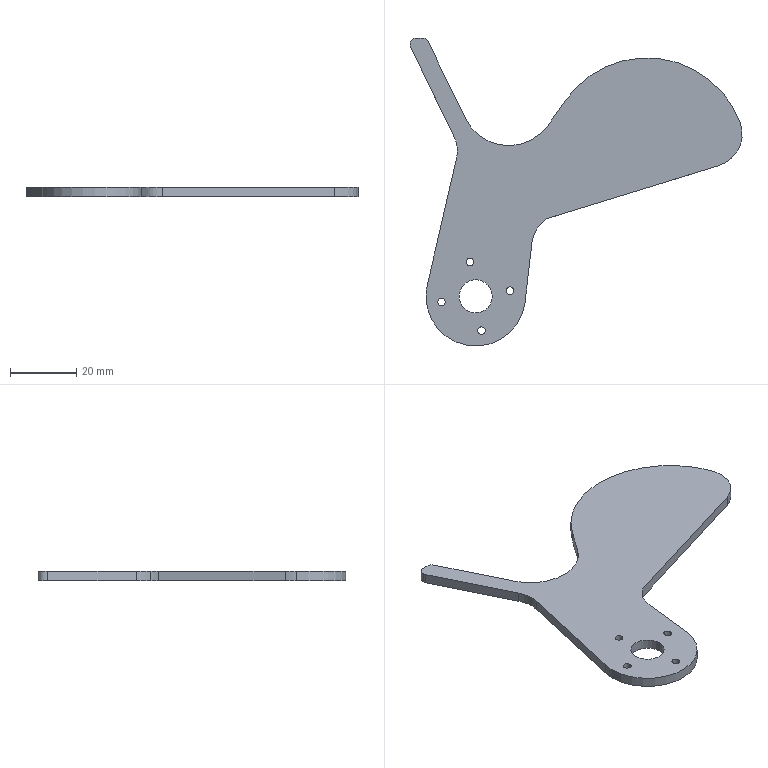Part | SolidWorks | features ICE 4, Fillet 2, BaseBody 1, HoleWzd 1 | 1 solid | 29 faces | box 100.288 x 93 x 3 mm | volume 11352 mm3 | cylinder 20 | plane 9 | commonest cylinder face diameters 2.3 x8 20 x4 4 x2 10 x2 30 x2 29 x1
STEP:
#1=CARTESIAN_POINT('',(-15.,-60.,0.));
#2=VERTEX_POINT('',#1);
#3=CARTESIAN_POINT('',(-5.,-60.,0.));
#4=VERTEX_POINT('',#3);
#5=CARTESIAN_POINT('',(-10.,-60.,0.));
#6=DIRECTION('',(0.,0.,1.));
#7=DIRECTION('',(1.,0.,0.));
#8=AXIS2_PLACEMENT_3D('',#5,#6,#7);
#9=CIRCLE('',#8,5.);
#10=EDGE_CURVE('',#2,#4,#9,.T.);
#11=ORIENTED_EDGE('',*,*,#10,.F.);
#12=CARTESIAN_POINT('',(-15.,-60.,3.));
#13=VERTEX_POINT('',#12);
#14=CARTESIAN_POINT('',(-15.,-60.,0.));
#15=DIRECTION('',(0.,0.,1.));
#16=VECTOR('',#15,1000.);
#17=LINE('',#14,#16);
#18=EDGE_CURVE('',#2,#13,#17,.T.);
#19=ORIENTED_EDGE('',*,*,#18,.T.);
#20=CARTESIAN_POINT('',(-5.,-60.,3.));
#21=VERTEX_POINT('',#20);
#22=CARTESIAN_POINT('',(-10.,-60.,3.));
#23=DIRECTION('',(0.,0.,1.));
#24=DIRECTION('',(1.,0.,0.));
#25=AXIS2_PLACEMENT_3D('',#22,#23,#24);
#26=CIRCLE('',#25,5.);
#27=EDGE_CURVE('',#13,#21,#26,.T.);
#28=ORIENTED_EDGE('',*,*,#27,.T.);
#29=CARTESIAN_POINT('',(-5.,-60.,0.));
#30=DIRECTION('',(0.,0.,1.));
#31=VECTOR('',#30,1000.);
#32=LINE('',#29,#31);
#33=EDGE_CURVE('',#4,#21,#32,.T.);
#34=ORIENTED_EDGE('',*,*,#33,.F.);
#35=EDGE_LOOP('',(#11,#19,#28,#34));
#36=FACE_OUTER_BOUND('',#35,.T.);
#37=CARTESIAN_POINT('',(-10.,-60.,0.));
#38=DIRECTION('',(0.,0.,1.));
#39=DIRECTION('',(1.,0.,0.));
#40=AXIS2_PLACEMENT_3D('',#37,#38,#39);
#41=CYLINDRICAL_SURFACE('',#40,5.);
#42=ADVANCED_FACE('',(#36),#41,.F.);
#43=CARTESIAN_POINT('',(-19.208,-61.722,0.));
#44=VERTEX_POINT('',#43);
#45=CARTESIAN_POINT('',(-21.508,-61.722,0.));
#46=VERTEX_POINT('',#45);
#47=CARTESIAN_POINT('',(-20.358,-61.722,0.));
#48=DIRECTION('',(0.,0.,-1.));
#49=DIRECTION('',(-1.,0.,0.));
#50=AXIS2_PLACEMENT_3D('',#47,#48,#49);
#51=CIRCLE('',#50,1.15);
#52=EDGE_CURVE('',#44,#46,#51,.T.);
#53=ORIENTED_EDGE('',*,*,#52,.T.);
#54=CARTESIAN_POINT('',(-21.508,-61.722,3.));
#55=VERTEX_POINT('',#54);
#56=CARTESIAN_POINT('',(-21.508,-61.722,3.));
#57=DIRECTION('',(0.,0.,1.));
#58=VECTOR('',#57,1000.);
#59=LINE('',#56,#58);
#60=EDGE_CURVE('',#46,#55,#59,.T.);
#61=ORIENTED_EDGE('',*,*,#60,.T.);
#62=CARTESIAN_POINT('',(-19.208,-61.722,3.));
#63=VERTEX_POINT('',#62);
#64=CARTESIAN_POINT('',(-20.358,-61.722,3.));
#65=DIRECTION('',(0.,0.,1.));
#66=DIRECTION('',(1.,0.,0.));
#67=AXIS2_PLACEMENT_3D('',#64,#65,#66);
#68=CIRCLE('',#67,1.15);
#69=EDGE_CURVE('',#55,#63,#68,.T.);
#70=ORIENTED_EDGE('',*,*,#69,.T.);
#71=CARTESIAN_POINT('',(-19.208,-61.722,3.));
#72=DIRECTION('',(0.,0.,1.));
#73=VECTOR('',#72,1000.);
#74=LINE('',#71,#73);
#75=EDGE_CURVE('',#44,#63,#74,.T.);
#76=ORIENTED_EDGE('',*,*,#75,.F.);
#77=EDGE_LOOP('',(#53,#61,#70,#76));
#78=FACE_OUTER_BOUND('',#77,.T.);
#79=CARTESIAN_POINT('',(-20.358,-61.722,3.));
#80=DIRECTION('',(0.,0.,1.));
#81=DIRECTION('',(1.,0.,0.));
#82=AXIS2_PLACEMENT_3D('',#79,#80,#81);
#83=CYLINDRICAL_SURFACE('',#82,1.15);
#84=ADVANCED_FACE('',(#78),#83,.F.);
#85=CARTESIAN_POINT('',(-10.572,-49.642,0.));
#86=VERTEX_POINT('',#85);
#87=CARTESIAN_POINT('',(-12.872,-49.642,0.));
#88=VERTEX_POINT('',#87);
#89=CARTESIAN_POINT('',(-11.722,-49.642,0.));
#90=DIRECTION('',(0.,0.,-1.));
#91=DIRECTION('',(-1.,0.,0.));
#92=AXIS2_PLACEMENT_3D('',#89,#90,#91);
#93=CIRCLE('',#92,1.15);
#94=EDGE_CURVE('',#86,#88,#93,.T.);
#95=ORIENTED_EDGE('',*,*,#94,.T.);
#96=CARTESIAN_POINT('',(-12.872,-49.642,3.));
#97=VERTEX_POINT('',#96);
#98=CARTESIAN_POINT('',(-12.872,-49.642,3.));
#99=DIRECTION('',(0.,0.,1.));
#100=VECTOR('',#99,1000.);
#101=LINE('',#98,#100);
#102=EDGE_CURVE('',#88,#97,#101,.T.);
#103=ORIENTED_EDGE('',*,*,#102,.T.);
#104=CARTESIAN_POINT('',(-10.572,-49.642,3.));
#105=VERTEX_POINT('',#104);
#106=CARTESIAN_POINT('',(-11.722,-49.642,3.));
#107=DIRECTION('',(0.,0.,1.));
#108=DIRECTION('',(1.,0.,0.));
#109=AXIS2_PLACEMENT_3D('',#106,#107,#108);
#110=CIRCLE('',#109,1.15);
#111=EDGE_CURVE('',#97,#105,#110,.T.);
#112=ORIENTED_EDGE('',*,*,#111,.T.);
#113=CARTESIAN_POINT('',(-10.572,-49.642,3.));
#114=DIRECTION('',(0.,0.,1.));
#115=VECTOR('',#114,1000.);
#116=LINE('',#113,#115);
#117=EDGE_CURVE('',#86,#105,#116,.T.);
#118=ORIENTED_EDGE('',*,*,#117,.F.);
#119=EDGE_LOOP('',(#95,#103,#112,#118));
#120=FACE_OUTER_BOUND('',#119,.T.);
#121=CARTESIAN_POINT('',(-11.722,-49.642,3.));
#122=DIRECTION('',(0.,0.,1.));
#123=DIRECTION('',(1.,0.,0.));
#124=AXIS2_PLACEMENT_3D('',#121,#122,#123);
#125=CYLINDRICAL_SURFACE('',#124,1.15);
#126=ADVANCED_FACE('',(#120),#125,.F.);
#127=CARTESIAN_POINT('',(-7.128,-70.358,0.));
#128=VERTEX_POINT('',#127);
#129=CARTESIAN_POINT('',(-9.428,-70.358,0.));
#130=VERTEX_POINT('',#129);
#131=CARTESIAN_POINT('',(-8.278,-70.358,0.));
#132=DIRECTION('',(0.,0.,-1.));
#133=DIRECTION('',(-1.,0.,0.));
#134=AXIS2_PLACEMENT_3D('',#131,#132,#133);
#135=CIRCLE('',#134,1.15);
#136=EDGE_CURVE('',#128,#130,#135,.T.);
#137=ORIENTED_EDGE('',*,*,#136,.T.);
#138=CARTESIAN_POINT('',(-9.428,-70.358,3.));
#139=VERTEX_POINT('',#138);
#140=CARTESIAN_POINT('',(-9.428,-70.358,3.));
#141=DIRECTION('',(0.,0.,1.));
#142=VECTOR('',#141,1000.);
#143=LINE('',#140,#142);
#144=EDGE_CURVE('',#130,#139,#143,.T.);
#145=ORIENTED_EDGE('',*,*,#144,.T.);
#146=CARTESIAN_POINT('',(-7.128,-70.358,3.));
#147=VERTEX_POINT('',#146);
#148=CARTESIAN_POINT('',(-8.278,-70.358,3.));
#149=DIRECTION('',(0.,0.,1.));
#150=DIRECTION('',(1.,0.,0.));
#151=AXIS2_PLACEMENT_3D('',#148,#149,#150);
#152=CIRCLE('',#151,1.15);
#153=EDGE_CURVE('',#139,#147,#152,.T.);
#154=ORIENTED_EDGE('',*,*,#153,.T.);
#155=CARTESIAN_POINT('',(-7.128,-70.358,3.));
#156=DIRECTION('',(0.,0.,1.));
#157=VECTOR('',#156,1000.);
#158=LINE('',#155,#157);
#159=EDGE_CURVE('',#128,#147,#158,.T.);
#160=ORIENTED_EDGE('',*,*,#159,.F.);
#161=EDGE_LOOP('',(#137,#145,#154,#160));
#162=FACE_OUTER_BOUND('',#161,.T.);
#163=CARTESIAN_POINT('',(-8.278,-70.358,3.));
#164=DIRECTION('',(0.,0.,1.));
#165=DIRECTION('',(1.,0.,0.));
#166=AXIS2_PLACEMENT_3D('',#163,#164,#165);
#167=CYLINDRICAL_SURFACE('',#166,1.15);
#168=ADVANCED_FACE('',(#162),#167,.F.);
#169=CARTESIAN_POINT('',(1.508,-58.278,0.));
#170=VERTEX_POINT('',#169);
#171=CARTESIAN_POINT('',(-0.7921,-58.278,0.));
#172=VERTEX_POINT('',#171);
#173=CARTESIAN_POINT('',(0.3579,-58.278,0.));
#174=DIRECTION('',(0.,0.,-1.));
#175=DIRECTION('',(-1.,0.,0.));
#176=AXIS2_PLACEMENT_3D('',#173,#174,#175);
#177=CIRCLE('',#176,1.15);
#178=EDGE_CURVE('',#170,#172,#177,.T.);
#179=ORIENTED_EDGE('',*,*,#178,.T.);
#180=CARTESIAN_POINT('',(-0.7921,-58.278,3.));
#181=VERTEX_POINT('',#180);
#182=CARTESIAN_POINT('',(-0.7921,-58.278,3.));
#183=DIRECTION('',(0.,0.,1.));
#184=VECTOR('',#183,1000.);
#185=LINE('',#182,#184);
#186=EDGE_CURVE('',#172,#181,#185,.T.);
#187=ORIENTED_EDGE('',*,*,#186,.T.);
#188=CARTESIAN_POINT('',(1.508,-58.278,3.));
#189=VERTEX_POINT('',#188);
#190=CARTESIAN_POINT('',(0.3579,-58.278,3.));
#191=DIRECTION('',(0.,0.,1.));
#192=DIRECTION('',(1.,0.,0.));
#193=AXIS2_PLACEMENT_3D('',#190,#191,#192);
#194=CIRCLE('',#193,1.15);
#195=EDGE_CURVE('',#181,#189,#194,.T.);
#196=ORIENTED_EDGE('',*,*,#195,.T.);
#197=CARTESIAN_POINT('',(1.508,-58.278,3.));
#198=DIRECTION('',(0.,0.,1.));
#199=VECTOR('',#198,1000.);
#200=LINE('',#197,#199);
#201=EDGE_CURVE('',#170,#189,#200,.T.);
#202=ORIENTED_EDGE('',*,*,#201,.F.);
#203=EDGE_LOOP('',(#179,#187,#196,#202));
#204=FACE_OUTER_BOUND('',#203,.T.);
#205=CARTESIAN_POINT('',(0.3579,-58.278,3.));
#206=DIRECTION('',(0.,0.,1.));
#207=DIRECTION('',(1.,0.,0.));
#208=AXIS2_PLACEMENT_3D('',#205,#206,#207);
#209=CYLINDRICAL_SURFACE('',#208,1.15);
#210=ADVANCED_FACE('',(#204),#209,.F.);
#211=CARTESIAN_POINT('',(-15.539,-16.073,0.));
#212=VERTEX_POINT('',#211);
#213=CARTESIAN_POINT('',(-16.551,-11.689,0.));
#214=VERTEX_POINT('',#213);
#215=CARTESIAN_POINT('',(-25.539,-16.073,0.));
#216=DIRECTION('',(0.,0.,1.));
#217=DIRECTION('',(1.,0.,0.));
#218=AXIS2_PLACEMENT_3D('',#215,#216,#217);
#219=CIRCLE('',#218,10.);
#220=EDGE_CURVE('',#212,#214,#219,.T.);
#221=ORIENTED_EDGE('',*,*,#220,.F.);
#222=CARTESIAN_POINT('',(-15.539,-16.073,3.));
#223=VERTEX_POINT('',#222);
#224=CARTESIAN_POINT('',(-15.539,-16.073,0.));
#225=DIRECTION('',(0.,0.,1.));
#226=VECTOR('',#225,1000.);
#227=LINE('',#224,#226);
#228=EDGE_CURVE('',#212,#223,#227,.T.);
#229=ORIENTED_EDGE('',*,*,#228,.T.);
#230=CARTESIAN_POINT('',(-16.551,-11.689,3.));
#231=VERTEX_POINT('',#230);
#232=CARTESIAN_POINT('',(-25.539,-16.073,3.));
#233=DIRECTION('',(0.,0.,-1.));
#234=DIRECTION('',(1.,0.,0.));
#235=AXIS2_PLACEMENT_3D('',#232,#233,#234);
#236=CIRCLE('',#235,10.);
#237=EDGE_CURVE('',#231,#223,#236,.T.);
#238=ORIENTED_EDGE('',*,*,#237,.F.);
#239=CARTESIAN_POINT('',(-16.551,-11.689,1.5));
#240=DIRECTION('',(0.,0.,1.));
#241=VECTOR('',#240,1000.);
#242=LINE('',#239,#241);
#243=EDGE_CURVE('',#214,#231,#242,.T.);
#244=ORIENTED_EDGE('',*,*,#243,.F.);
#245=EDGE_LOOP('',(#221,#229,#238,#244));
#246=FACE_OUTER_BOUND('',#245,.T.);
#247=CARTESIAN_POINT('',(-25.539,-16.073,0.));
#248=DIRECTION('',(0.,0.,1.));
#249=DIRECTION('',(1.,0.,0.));
#250=AXIS2_PLACEMENT_3D('',#247,#248,#249);
#251=CYLINDRICAL_SURFACE('',#250,10.);
#252=ADVANCED_FACE('',(#246),#251,.F.);
#253=CARTESIAN_POINT('',(-25.,-60.,3.));
#254=VERTEX_POINT('',#253);
#255=CARTESIAN_POINT('',(4.9,-61.728,3.));
#256=VERTEX_POINT('',#255);
#257=CARTESIAN_POINT('',(-10.,-60.,3.));
#258=DIRECTION('',(0.,0.,1.));
#259=DIRECTION('',(-1.,0.,0.));
#260=AXIS2_PLACEMENT_3D('',#257,#258,#259);
#261=CIRCLE('',#260,15.);
#262=EDGE_CURVE('',#254,#256,#261,.T.);
#263=ORIENTED_EDGE('',*,*,#262,.F.);
#264=CARTESIAN_POINT('',(-25.,-60.,0.));
#265=VERTEX_POINT('',#264);
#266=CARTESIAN_POINT('',(-25.,-60.,3.));
#267=DIRECTION('',(0.,0.,-1.));
#268=VECTOR('',#267,1000.);
#269=LINE('',#266,#268);
#270=EDGE_CURVE('',#254,#265,#269,.T.);
#271=ORIENTED_EDGE('',*,*,#270,.T.);
#272=CARTESIAN_POINT('',(4.9,-61.728,0.));
#273=VERTEX_POINT('',#272);
#274=CARTESIAN_POINT('',(-10.,-60.,0.));
#275=DIRECTION('',(0.,0.,-1.));
#276=DIRECTION('',(-1.,0.,0.));
#277=AXIS2_PLACEMENT_3D('',#274,#275,#276);
#278=CIRCLE('',#277,15.);
#279=EDGE_CURVE('',#273,#265,#278,.T.);
#280=ORIENTED_EDGE('',*,*,#279,.F.);
#281=CARTESIAN_POINT('',(4.9,-61.728,1.5));
#282=DIRECTION('',(0.,0.,1.));
#283=VECTOR('',#282,1000.);
#284=LINE('',#281,#283);
#285=EDGE_CURVE('',#273,#256,#284,.T.);
#286=ORIENTED_EDGE('',*,*,#285,.T.);
#287=EDGE_LOOP('',(#263,#271,#280,#286));
#288=FACE_OUTER_BOUND('',#287,.T.);
#289=CARTESIAN_POINT('',(-10.,-60.,3.));
#290=DIRECTION('',(0.,0.,-1.));
#291=DIRECTION('',(-1.,0.,0.));
#292=AXIS2_PLACEMENT_3D('',#289,#290,#291);
#293=CYLINDRICAL_SURFACE('',#292,15.);
#294=ADVANCED_FACE('',(#288),#293,.T.);
#295=CARTESIAN_POINT('',(-10.,-60.,3.));
#296=DIRECTION('',(0.,0.,1.));
#297=DIRECTION('',(1.,0.,0.));
#298=AXIS2_PLACEMENT_3D('',#295,#296,#297);
#299=CIRCLE('',#298,5.);
#300=EDGE_CURVE('',#21,#13,#299,.T.);
#301=ORIENTED_EDGE('',*,*,#300,.F.);
#302=ORIENTED_EDGE('',*,*,#27,.F.);
#303=EDGE_LOOP('',(#301,#302));
#304=FACE_BOUND('',#303,.T.);
#305=CARTESIAN_POINT('',(-20.358,-61.722,3.));
#306=DIRECTION('',(0.,0.,1.));
#307=DIRECTION('',(1.,0.,0.));
#308=AXIS2_PLACEMENT_3D('',#305,#306,#307);
#309=CIRCLE('',#308,1.15);
#310=EDGE_CURVE('',#63,#55,#309,.T.);
#311=ORIENTED_EDGE('',*,*,#310,.F.);
#312=ORIENTED_EDGE('',*,*,#69,.F.);
#313=EDGE_LOOP('',(#311,#312));
#314=FACE_BOUND('',#313,.T.);
#315=CARTESIAN_POINT('',(-11.722,-49.642,3.));
#316=DIRECTION('',(0.,0.,1.));
#317=DIRECTION('',(1.,0.,0.));
#318=AXIS2_PLACEMENT_3D('',#315,#316,#317);
#319=CIRCLE('',#318,1.15);
#320=EDGE_CURVE('',#105,#97,#319,.T.);
#321=ORIENTED_EDGE('',*,*,#320,.F.);
#322=ORIENTED_EDGE('',*,*,#111,.F.);
#323=EDGE_LOOP('',(#321,#322));
#324=FACE_BOUND('',#323,.T.);
#325=CARTESIAN_POINT('',(-8.278,-70.358,3.));
#326=DIRECTION('',(0.,0.,1.));
#327=DIRECTION('',(1.,0.,0.));
#328=AXIS2_PLACEMENT_3D('',#325,#326,#327);
#329=CIRCLE('',#328,1.15);
#330=EDGE_CURVE('',#147,#139,#329,.T.);
#331=ORIENTED_EDGE('',*,*,#330,.F.);
#332=ORIENTED_EDGE('',*,*,#153,.F.);
#333=EDGE_LOOP('',(#331,#332));
#334=FACE_BOUND('',#333,.T.);
#335=CARTESIAN_POINT('',(0.3579,-58.278,3.));
#336=DIRECTION('',(0.,0.,1.));
#337=DIRECTION('',(1.,0.,0.));
#338=AXIS2_PLACEMENT_3D('',#335,#336,#337);
#339=CIRCLE('',#338,1.15);
#340=EDGE_CURVE('',#189,#181,#339,.T.);
#341=ORIENTED_EDGE('',*,*,#340,.F.);
#342=ORIENTED_EDGE('',*,*,#195,.F.);
#343=EDGE_LOOP('',(#341,#342));
#344=FACE_BOUND('',#343,.T.);
#345=CARTESIAN_POINT('',(63.401,-20.562,3.));
#346=VERTEX_POINT('',#345);
#347=CARTESIAN_POINT('',(11.431,-36.568,3.));
#348=VERTEX_POINT('',#347);
#349=CARTESIAN_POINT('',(11.276,-36.615,3.));
#350=DIRECTION('',(-0.9557,-0.2943,0.));
#351=VECTOR('',#350,1000.);
#352=LINE('',#349,#351);
#353=EDGE_CURVE('',#346,#348,#352,.T.);
#354=ORIENTED_EDGE('',*,*,#353,.F.);
#355=CARTESIAN_POINT('',(69.826,-7.508,3.));
#356=VERTEX_POINT('',#355);
#357=CARTESIAN_POINT('',(60.458,-11.005,3.));
#358=DIRECTION('',(0.,0.,1.));
#359=DIRECTION('',(1.,0.,0.));
#360=AXIS2_PLACEMENT_3D('',#357,#358,#359);
#361=CIRCLE('',#360,10.);
#362=EDGE_CURVE('',#346,#356,#361,.T.);
#363=ORIENTED_EDGE('',*,*,#362,.T.);
#364=CARTESIAN_POINT('',(17.146,-0.7927,3.));
#365=VERTEX_POINT('',#364);
#366=CARTESIAN_POINT('',(41.721,-18.,3.));
#367=DIRECTION('',(0.,0.,1.));
#368=DIRECTION('',(-1.,0.,0.));
#369=AXIS2_PLACEMENT_3D('',#366,#367,#368);
#370=CIRCLE('',#369,30.);
#371=EDGE_CURVE('',#356,#365,#370,.T.);
#372=ORIENTED_EDGE('',*,*,#371,.T.);
#373=CARTESIAN_POINT('',(11.878,-8.317,3.));
#374=VERTEX_POINT('',#373);
#375=CARTESIAN_POINT('',(17.146,-0.7927,3.));
#376=DIRECTION('',(-0.5736,-0.8192,0.));
#377=VECTOR('',#376,1000.);
#378=LINE('',#375,#377);
#379=EDGE_CURVE('',#365,#374,#378,.T.);
#380=ORIENTED_EDGE('',*,*,#379,.T.);
#381=CARTESIAN_POINT('',(-13.033,-6.356,3.));
#382=VERTEX_POINT('',#381);
#383=CARTESIAN_POINT('',(0.,0.,3.));
#384=DIRECTION('',(0.,0.,-1.));
#385=DIRECTION('',(1.,0.,0.));
#386=AXIS2_PLACEMENT_3D('',#383,#384,#385);
#387=CIRCLE('',#386,14.5);
#388=EDGE_CURVE('',#374,#382,#387,.T.);
#389=ORIENTED_EDGE('',*,*,#388,.T.);
#390=CARTESIAN_POINT('',(-24.364,16.877,3.));
#391=VERTEX_POINT('',#390);
#392=CARTESIAN_POINT('',(-13.033,-6.356,3.));
#393=DIRECTION('',(-0.4384,0.8988,0.));
#394=VECTOR('',#393,1000.);
#395=LINE('',#392,#394);
#396=EDGE_CURVE('',#382,#391,#395,.T.);
#397=ORIENTED_EDGE('',*,*,#396,.T.);
#398=CARTESIAN_POINT('',(-26.162,18.,3.));
#399=VERTEX_POINT('',#398);
#400=CARTESIAN_POINT('',(-26.162,16.,3.));
#401=DIRECTION('',(0.,0.,1.));
#402=DIRECTION('',(0.,1.,0.));
#403=AXIS2_PLACEMENT_3D('',#400,#401,#402);
#404=CIRCLE('',#403,2.);
#405=EDGE_CURVE('',#391,#399,#404,.T.);
#406=ORIENTED_EDGE('',*,*,#405,.T.);
#407=CARTESIAN_POINT('',(-27.831,18.,3.));
#408=VERTEX_POINT('',#407);
#409=CARTESIAN_POINT('',(-26.996,18.,3.));
#410=DIRECTION('',(1.,0.,0.));
#411=VECTOR('',#410,1000.);
#412=LINE('',#409,#411);
#413=EDGE_CURVE('',#408,#399,#412,.T.);
#414=ORIENTED_EDGE('',*,*,#413,.F.);
#415=CARTESIAN_POINT('',(-29.628,15.123,3.));
#416=VERTEX_POINT('',#415);
#417=CARTESIAN_POINT('',(-27.831,16.,3.));
#418=DIRECTION('',(0.,0.,1.));
#419=DIRECTION('',(0.,1.,0.));
#420=AXIS2_PLACEMENT_3D('',#417,#418,#419);
#421=CIRCLE('',#420,2.);
#422=EDGE_CURVE('',#408,#416,#421,.T.);
#423=ORIENTED_EDGE('',*,*,#422,.T.);
#424=CARTESIAN_POINT('',(-29.628,15.123,3.));
#425=DIRECTION('',(0.4384,-0.8988,0.));
#426=VECTOR('',#425,1000.);
#427=LINE('',#424,#426);
#428=EDGE_CURVE('',#416,#231,#427,.T.);
#429=ORIENTED_EDGE('',*,*,#428,.T.);
#430=ORIENTED_EDGE('',*,*,#237,.T.);
#431=CARTESIAN_POINT('',(-15.794,-18.317,3.));
#432=VERTEX_POINT('',#431);
#433=CARTESIAN_POINT('',(-25.539,-16.073,3.));
#434=DIRECTION('',(0.,0.,-1.));
#435=DIRECTION('',(1.,0.,0.));
#436=AXIS2_PLACEMENT_3D('',#433,#434,#435);
#437=CIRCLE('',#436,10.);
#438=EDGE_CURVE('',#223,#432,#437,.T.);
#439=ORIENTED_EDGE('',*,*,#438,.T.);
#440=CARTESIAN_POINT('',(-24.617,-56.634,3.));
#441=VERTEX_POINT('',#440);
#442=CARTESIAN_POINT('',(-15.794,-18.317,3.));
#443=DIRECTION('',(-0.2244,-0.9745,0.));
#444=VECTOR('',#443,1000.);
#445=LINE('',#442,#444);
#446=EDGE_CURVE('',#432,#441,#445,.T.);
#447=ORIENTED_EDGE('',*,*,#446,.T.);
#448=CARTESIAN_POINT('',(-10.,-60.,3.));
#449=DIRECTION('',(0.,0.,1.));
#450=DIRECTION('',(-1.,0.,0.));
#451=AXIS2_PLACEMENT_3D('',#448,#449,#450);
#452=CIRCLE('',#451,15.);
#453=EDGE_CURVE('',#441,#254,#452,.T.);
#454=ORIENTED_EDGE('',*,*,#453,.T.);
#455=ORIENTED_EDGE('',*,*,#262,.T.);
#456=CARTESIAN_POINT('',(6.982,-43.777,3.));
#457=VERTEX_POINT('',#456);
#458=CARTESIAN_POINT('',(4.9,-61.728,3.));
#459=DIRECTION('',(0.1152,0.9933,0.));
#460=VECTOR('',#459,1000.);
#461=LINE('',#458,#460);
#462=EDGE_CURVE('',#256,#457,#461,.T.);
#463=ORIENTED_EDGE('',*,*,#462,.T.);
#464=CARTESIAN_POINT('',(16.915,-44.929,3.));
#465=DIRECTION('',(0.,0.,-1.));
#466=DIRECTION('',(1.,0.,0.));
#467=AXIS2_PLACEMENT_3D('',#464,#465,#466);
#468=CIRCLE('',#467,10.);
#469=EDGE_CURVE('',#457,#348,#468,.T.);
#470=ORIENTED_EDGE('',*,*,#469,.T.);
#471=EDGE_LOOP('',(#354,#363,#372,#380,#389,#397,#406,#414,#423,#429,#430,#439,#447,#454,#455,#463,#470));
#472=FACE_OUTER_BOUND('',#471,.T.);
#473=CARTESIAN_POINT('',(-30.124,-77.265,3.));
#474=DIRECTION('',(0.,0.,1.));
#475=DIRECTION('',(1.,0.,0.));
#476=AXIS2_PLACEMENT_3D('',#473,#474,#475);
#477=PLANE('',#476);
#478=ADVANCED_FACE('',(#304,#314,#324,#334,#344,#472),#477,.T.);
#479=CARTESIAN_POINT('',(-10.,-60.,0.));
#480=DIRECTION('',(0.,0.,1.));
#481=DIRECTION('',(1.,0.,0.));
#482=AXIS2_PLACEMENT_3D('',#479,#480,#481);
#483=CIRCLE('',#482,5.);
#484=EDGE_CURVE('',#4,#2,#483,.T.);
#485=ORIENTED_EDGE('',*,*,#484,.T.);
#486=ORIENTED_EDGE('',*,*,#10,.T.);
#487=EDGE_LOOP('',(#485,#486));
#488=FACE_BOUND('',#487,.T.);
#489=ORIENTED_EDGE('',*,*,#52,.F.);
#490=CARTESIAN_POINT('',(-20.358,-61.722,0.));
#491=DIRECTION('',(0.,0.,-1.));
#492=DIRECTION('',(-1.,0.,0.));
#493=AXIS2_PLACEMENT_3D('',#490,#491,#492);
#494=CIRCLE('',#493,1.15);
#495=EDGE_CURVE('',#46,#44,#494,.T.);
#496=ORIENTED_EDGE('',*,*,#495,.F.);
#497=EDGE_LOOP('',(#489,#496));
#498=FACE_BOUND('',#497,.T.);
#499=ORIENTED_EDGE('',*,*,#94,.F.);
#500=CARTESIAN_POINT('',(-11.722,-49.642,0.));
#501=DIRECTION('',(0.,0.,-1.));
#502=DIRECTION('',(-1.,0.,0.));
#503=AXIS2_PLACEMENT_3D('',#500,#501,#502);
#504=CIRCLE('',#503,1.15);
#505=EDGE_CURVE('',#88,#86,#504,.T.);
#506=ORIENTED_EDGE('',*,*,#505,.F.);
#507=EDGE_LOOP('',(#499,#506));
#508=FACE_BOUND('',#507,.T.);
#509=ORIENTED_EDGE('',*,*,#136,.F.);
#510=CARTESIAN_POINT('',(-8.278,-70.358,0.));
#511=DIRECTION('',(0.,0.,-1.));
#512=DIRECTION('',(-1.,0.,0.));
#513=AXIS2_PLACEMENT_3D('',#510,#511,#512);
#514=CIRCLE('',#513,1.15);
#515=EDGE_CURVE('',#130,#128,#514,.T.);
#516=ORIENTED_EDGE('',*,*,#515,.F.);
#517=EDGE_LOOP('',(#509,#516));
#518=FACE_BOUND('',#517,.T.);
#519=ORIENTED_EDGE('',*,*,#178,.F.);
#520=CARTESIAN_POINT('',(0.3579,-58.278,0.));
#521=DIRECTION('',(0.,0.,-1.));
#522=DIRECTION('',(-1.,0.,0.));
#523=AXIS2_PLACEMENT_3D('',#520,#521,#522);
#524=CIRCLE('',#523,1.15);
#525=EDGE_CURVE('',#172,#170,#524,.T.);
#526=ORIENTED_EDGE('',*,*,#525,.F.);
#527=EDGE_LOOP('',(#519,#526));
#528=FACE_BOUND('',#527,.T.);
#529=CARTESIAN_POINT('',(17.146,-0.7927,0.));
#530=VERTEX_POINT('',#529);
#531=CARTESIAN_POINT('',(69.826,-7.508,0.));
#532=VERTEX_POINT('',#531);
#533=CARTESIAN_POINT('',(41.721,-18.,0.));
#534=DIRECTION('',(0.,0.,-1.));
#535=DIRECTION('',(-1.,0.,0.));
#536=AXIS2_PLACEMENT_3D('',#533,#534,#535);
#537=CIRCLE('',#536,30.);
#538=EDGE_CURVE('',#530,#532,#537,.T.);
#539=ORIENTED_EDGE('',*,*,#538,.T.);
#540=CARTESIAN_POINT('',(63.401,-20.562,0.));
#541=VERTEX_POINT('',#540);
#542=CARTESIAN_POINT('',(60.458,-11.005,0.));
#543=DIRECTION('',(0.,0.,-1.));
#544=DIRECTION('',(-1.,0.,0.));
#545=AXIS2_PLACEMENT_3D('',#542,#543,#544);
#546=CIRCLE('',#545,10.);
#547=EDGE_CURVE('',#532,#541,#546,.T.);
#548=ORIENTED_EDGE('',*,*,#547,.T.);
#549=CARTESIAN_POINT('',(11.431,-36.568,0.));
#550=VERTEX_POINT('',#549);
#551=CARTESIAN_POINT('',(11.276,-36.615,0.));
#552=DIRECTION('',(-0.9557,-0.2943,0.));
#553=VECTOR('',#552,1000.);
#554=LINE('',#551,#553);
#555=EDGE_CURVE('',#541,#550,#554,.T.);
#556=ORIENTED_EDGE('',*,*,#555,.T.);
#557=CARTESIAN_POINT('',(6.982,-43.777,0.));
#558=VERTEX_POINT('',#557);
#559=CARTESIAN_POINT('',(16.915,-44.929,0.));
#560=DIRECTION('',(0.,0.,1.));
#561=DIRECTION('',(-1.,0.,0.));
#562=AXIS2_PLACEMENT_3D('',#559,#560,#561);
#563=CIRCLE('',#562,10.);
#564=EDGE_CURVE('',#550,#558,#563,.T.);
#565=ORIENTED_EDGE('',*,*,#564,.T.);
#566=CARTESIAN_POINT('',(7.521,-39.132,0.));
#567=DIRECTION('',(-0.1152,-0.9933,0.));
#568=VECTOR('',#567,1000.);
#569=LINE('',#566,#568);
#570=EDGE_CURVE('',#558,#273,#569,.T.);
#571=ORIENTED_EDGE('',*,*,#570,.T.);
#572=ORIENTED_EDGE('',*,*,#279,.T.);
#573=CARTESIAN_POINT('',(-24.617,-56.634,0.));
#574=VERTEX_POINT('',#573);
#575=CARTESIAN_POINT('',(-10.,-60.,0.));
#576=DIRECTION('',(0.,0.,-1.));
#577=DIRECTION('',(-1.,0.,0.));
#578=AXIS2_PLACEMENT_3D('',#575,#576,#577);
#579=CIRCLE('',#578,15.);
#580=EDGE_CURVE('',#265,#574,#579,.T.);
#581=ORIENTED_EDGE('',*,*,#580,.T.);
#582=CARTESIAN_POINT('',(-15.794,-18.317,0.));
#583=VERTEX_POINT('',#582);
#584=CARTESIAN_POINT('',(-24.617,-56.634,0.));
#585=DIRECTION('',(0.2244,0.9745,0.));
#586=VECTOR('',#585,1000.);
#587=LINE('',#584,#586);
#588=EDGE_CURVE('',#574,#583,#587,.T.);
#589=ORIENTED_EDGE('',*,*,#588,.T.);
#590=CARTESIAN_POINT('',(-25.539,-16.073,0.));
#591=DIRECTION('',(0.,0.,1.));
#592=DIRECTION('',(1.,0.,0.));
#593=AXIS2_PLACEMENT_3D('',#590,#591,#592);
#594=CIRCLE('',#593,10.);
#595=EDGE_CURVE('',#583,#212,#594,.T.);
#596=ORIENTED_EDGE('',*,*,#595,.T.);
#597=ORIENTED_EDGE('',*,*,#220,.T.);
#598=CARTESIAN_POINT('',(-29.628,15.123,0.));
#599=VERTEX_POINT('',#598);
#600=CARTESIAN_POINT('',(-16.551,-11.689,0.));
#601=DIRECTION('',(-0.4384,0.8988,0.));
#602=VECTOR('',#601,1000.);
#603=LINE('',#600,#602);
#604=EDGE_CURVE('',#214,#599,#603,.T.);
#605=ORIENTED_EDGE('',*,*,#604,.T.);
#606=CARTESIAN_POINT('',(-27.831,18.,0.));
#607=VERTEX_POINT('',#606);
#608=CARTESIAN_POINT('',(-27.831,16.,0.));
#609=DIRECTION('',(0.,0.,-1.));
#610=DIRECTION('',(0.,1.,0.));
#611=AXIS2_PLACEMENT_3D('',#608,#609,#610);
#612=CIRCLE('',#611,2.);
#613=EDGE_CURVE('',#599,#607,#612,.T.);
#614=ORIENTED_EDGE('',*,*,#613,.T.);
#615=CARTESIAN_POINT('',(-26.162,18.,0.));
#616=VERTEX_POINT('',#615);
#617=CARTESIAN_POINT('',(-26.996,18.,0.));
#618=DIRECTION('',(-1.,0.,0.));
#619=VECTOR('',#618,1000.);
#620=LINE('',#617,#619);
#621=EDGE_CURVE('',#616,#607,#620,.T.);
#622=ORIENTED_EDGE('',*,*,#621,.F.);
#623=CARTESIAN_POINT('',(-24.364,16.877,0.));
#624=VERTEX_POINT('',#623);
#625=CARTESIAN_POINT('',(-26.162,16.,0.));
#626=DIRECTION('',(0.,0.,-1.));
#627=DIRECTION('',(0.,1.,0.));
#628=AXIS2_PLACEMENT_3D('',#625,#626,#627);
#629=CIRCLE('',#628,2.);
#630=EDGE_CURVE('',#616,#624,#629,.T.);
#631=ORIENTED_EDGE('',*,*,#630,.T.);
#632=CARTESIAN_POINT('',(-13.033,-6.356,0.));
#633=VERTEX_POINT('',#632);
#634=CARTESIAN_POINT('',(-24.364,16.877,0.));
#635=DIRECTION('',(0.4384,-0.8988,0.));
#636=VECTOR('',#635,1000.);
#637=LINE('',#634,#636);
#638=EDGE_CURVE('',#624,#633,#637,.T.);
#639=ORIENTED_EDGE('',*,*,#638,.T.);
#640=CARTESIAN_POINT('',(11.878,-8.317,0.));
#641=VERTEX_POINT('',#640);
#642=CARTESIAN_POINT('',(0.,0.,0.));
#643=DIRECTION('',(0.,0.,1.));
#644=DIRECTION('',(1.,0.,0.));
#645=AXIS2_PLACEMENT_3D('',#642,#643,#644);
#646=CIRCLE('',#645,14.5);
#647=EDGE_CURVE('',#633,#641,#646,.T.);
#648=ORIENTED_EDGE('',*,*,#647,.T.);
#649=CARTESIAN_POINT('',(11.878,-8.317,0.));
#650=DIRECTION('',(0.5736,0.8192,0.));
#651=VECTOR('',#650,1000.);
#652=LINE('',#649,#651);
#653=EDGE_CURVE('',#641,#530,#652,.T.);
#654=ORIENTED_EDGE('',*,*,#653,.T.);
#655=EDGE_LOOP('',(#539,#548,#556,#565,#571,#572,#581,#589,#596,#597,#605,#614,#622,#631,#639,#648,#654));
#656=FACE_OUTER_BOUND('',#655,.T.);
#657=CARTESIAN_POINT('',(55.01,-77.265,0.));
#658=DIRECTION('',(0.,0.,-1.));
#659=DIRECTION('',(-1.,0.,0.));
#660=AXIS2_PLACEMENT_3D('',#657,#658,#659);
#661=PLANE('',#660);
#662=ADVANCED_FACE('',(#488,#498,#508,#518,#528,#656),#661,.T.);
#663=CARTESIAN_POINT('',(-29.628,15.123,1.5));
#664=DIRECTION('',(0.,0.,-1.));
#665=VECTOR('',#664,1000.);
#666=LINE('',#663,#665);
#667=EDGE_CURVE('',#416,#599,#666,.T.);
#668=ORIENTED_EDGE('',*,*,#667,.T.);
#669=ORIENTED_EDGE('',*,*,#604,.F.);
#670=ORIENTED_EDGE('',*,*,#243,.T.);
#671=ORIENTED_EDGE('',*,*,#428,.F.);
#672=EDGE_LOOP('',(#668,#669,#670,#671));
#673=FACE_OUTER_BOUND('',#672,.T.);
#674=CARTESIAN_POINT('',(-29.633,15.132,-0.01));
#675=DIRECTION('',(-0.8988,-0.4384,0.));
#676=DIRECTION('',(0.4384,-0.8988,0.));
#677=AXIS2_PLACEMENT_3D('',#674,#675,#676);
#678=PLANE('',#677);
#679=ADVANCED_FACE('',(#673),#678,.T.);
#680=ORIENTED_EDGE('',*,*,#228,.F.);
#681=ORIENTED_EDGE('',*,*,#595,.F.);
#682=CARTESIAN_POINT('',(-15.794,-18.317,1.5));
#683=DIRECTION('',(0.,0.,1.));
#684=VECTOR('',#683,1000.);
#685=LINE('',#682,#684);
#686=EDGE_CURVE('',#583,#432,#685,.T.);
#687=ORIENTED_EDGE('',*,*,#686,.T.);
#688=ORIENTED_EDGE('',*,*,#438,.F.);
#689=EDGE_LOOP('',(#680,#681,#687,#688));
#690=FACE_OUTER_BOUND('',#689,.T.);
#691=CARTESIAN_POINT('',(-25.539,-16.073,0.));
#692=DIRECTION('',(0.,0.,1.));
#693=DIRECTION('',(1.,0.,0.));
#694=AXIS2_PLACEMENT_3D('',#691,#692,#693);
#695=CYLINDRICAL_SURFACE('',#694,10.);
#696=ADVANCED_FACE('',(#690),#695,.F.);
#697=CARTESIAN_POINT('',(-24.617,-56.634,1.5));
#698=DIRECTION('',(0.,0.,1.));
#699=VECTOR('',#698,1000.);
#700=LINE('',#697,#699);
#701=EDGE_CURVE('',#574,#441,#700,.T.);
#702=ORIENTED_EDGE('',*,*,#701,.T.);
#703=ORIENTED_EDGE('',*,*,#446,.F.);
#704=ORIENTED_EDGE('',*,*,#686,.F.);
#705=ORIENTED_EDGE('',*,*,#588,.F.);
#706=EDGE_LOOP('',(#702,#703,#704,#705));
#707=FACE_OUTER_BOUND('',#706,.T.);
#708=CARTESIAN_POINT('',(-15.792,-18.307,-0.01));
#709=DIRECTION('',(-0.9745,0.2244,0.));
#710=DIRECTION('',(-0.2244,-0.9745,0.));
#711=AXIS2_PLACEMENT_3D('',#708,#709,#710);
#712=PLANE('',#711);
#713=ADVANCED_FACE('',(#707),#712,.T.);
#714=ORIENTED_EDGE('',*,*,#270,.F.);
#715=ORIENTED_EDGE('',*,*,#453,.F.);
#716=ORIENTED_EDGE('',*,*,#701,.F.);
#717=ORIENTED_EDGE('',*,*,#580,.F.);
#718=EDGE_LOOP('',(#714,#715,#716,#717));
#719=FACE_OUTER_BOUND('',#718,.T.);
#720=CARTESIAN_POINT('',(-10.,-60.,3.));
#721=DIRECTION('',(0.,0.,-1.));
#722=DIRECTION('',(-1.,0.,0.));
#723=AXIS2_PLACEMENT_3D('',#720,#721,#722);
#724=CYLINDRICAL_SURFACE('',#723,15.);
#725=ADVANCED_FACE('',(#719),#724,.T.);
#726=ORIENTED_EDGE('',*,*,#570,.F.);
#727=CARTESIAN_POINT('',(6.982,-43.777,3.));
#728=DIRECTION('',(0.,0.,1.));
#729=VECTOR('',#728,1000.);
#730=LINE('',#727,#729);
#731=EDGE_CURVE('',#558,#457,#730,.T.);
#732=ORIENTED_EDGE('',*,*,#731,.T.);
#733=ORIENTED_EDGE('',*,*,#462,.F.);
#734=ORIENTED_EDGE('',*,*,#285,.F.);
#735=EDGE_LOOP('',(#726,#732,#733,#734));
#736=FACE_OUTER_BOUND('',#735,.T.);
#737=CARTESIAN_POINT('',(4.899,-61.738,-0.01));
#738=DIRECTION('',(0.9933,-0.1152,0.));
#739=DIRECTION('',(0.1152,0.9933,0.));
#740=AXIS2_PLACEMENT_3D('',#737,#738,#739);
#741=PLANE('',#740);
#742=ADVANCED_FACE('',(#736),#741,.T.);
#743=ORIENTED_EDGE('',*,*,#371,.F.);
#744=CARTESIAN_POINT('',(69.826,-7.508,3.));
#745=DIRECTION('',(0.,0.,-1.));
#746=VECTOR('',#745,1000.);
#747=LINE('',#744,#746);
#748=EDGE_CURVE('',#356,#532,#747,.T.);
#749=ORIENTED_EDGE('',*,*,#748,.T.);
#750=ORIENTED_EDGE('',*,*,#538,.F.);
#751=CARTESIAN_POINT('',(17.146,-0.7927,1.5));
#752=DIRECTION('',(0.,0.,1.));
#753=VECTOR('',#752,1000.);
#754=LINE('',#751,#753);
#755=EDGE_CURVE('',#530,#365,#754,.T.);
#756=ORIENTED_EDGE('',*,*,#755,.T.);
#757=EDGE_LOOP('',(#743,#749,#750,#756));
#758=FACE_OUTER_BOUND('',#757,.T.);
#759=CARTESIAN_POINT('',(41.721,-18.,3.));
#760=DIRECTION('',(0.,0.,-1.));
#761=DIRECTION('',(-1.,0.,0.));
#762=AXIS2_PLACEMENT_3D('',#759,#760,#761);
#763=CYLINDRICAL_SURFACE('',#762,30.);
#764=ADVANCED_FACE('',(#758),#763,.T.);
#765=CARTESIAN_POINT('',(11.878,-8.317,1.5));
#766=DIRECTION('',(0.,0.,1.));
#767=VECTOR('',#766,1000.);
#768=LINE('',#765,#767);
#769=EDGE_CURVE('',#641,#374,#768,.T.);
#770=ORIENTED_EDGE('',*,*,#769,.T.);
#771=ORIENTED_EDGE('',*,*,#379,.F.);
#772=ORIENTED_EDGE('',*,*,#755,.F.);
#773=ORIENTED_EDGE('',*,*,#653,.F.);
#774=EDGE_LOOP('',(#770,#771,#772,#773));
#775=FACE_OUTER_BOUND('',#774,.T.);
#776=CARTESIAN_POINT('',(17.152,-0.7845,-0.01));
#777=DIRECTION('',(-0.8192,0.5736,0.));
#778=DIRECTION('',(-0.5736,-0.8192,0.));
#779=AXIS2_PLACEMENT_3D('',#776,#777,#778);
#780=PLANE('',#779);
#781=ADVANCED_FACE('',(#775),#780,.T.);
#782=ORIENTED_EDGE('',*,*,#388,.F.);
#783=ORIENTED_EDGE('',*,*,#769,.F.);
#784=ORIENTED_EDGE('',*,*,#647,.F.);
#785=CARTESIAN_POINT('',(-13.033,-6.356,1.5));
#786=DIRECTION('',(0.,0.,1.));
#787=VECTOR('',#786,1000.);
#788=LINE('',#785,#787);
#789=EDGE_CURVE('',#633,#382,#788,.T.);
#790=ORIENTED_EDGE('',*,*,#789,.T.);
#791=EDGE_LOOP('',(#782,#783,#784,#790));
#792=FACE_OUTER_BOUND('',#791,.T.);
#793=CARTESIAN_POINT('',(0.,0.,0.));
#794=DIRECTION('',(0.,0.,1.));
#795=DIRECTION('',(1.,0.,0.));
#796=AXIS2_PLACEMENT_3D('',#793,#794,#795);
#797=CYLINDRICAL_SURFACE('',#796,14.5);
#798=ADVANCED_FACE('',(#792),#797,.F.);
#799=ORIENTED_EDGE('',*,*,#789,.F.);
#800=ORIENTED_EDGE('',*,*,#638,.F.);
#801=CARTESIAN_POINT('',(-24.364,16.877,1.5));
#802=DIRECTION('',(0.,0.,1.));
#803=VECTOR('',#802,1000.);
#804=LINE('',#801,#803);
#805=EDGE_CURVE('',#624,#391,#804,.T.);
#806=ORIENTED_EDGE('',*,*,#805,.T.);
#807=ORIENTED_EDGE('',*,*,#396,.F.);
#808=EDGE_LOOP('',(#799,#800,#806,#807));
#809=FACE_OUTER_BOUND('',#808,.T.);
#810=CARTESIAN_POINT('',(-13.028,-6.365,-0.01));
#811=DIRECTION('',(0.8988,0.4384,0.));
#812=DIRECTION('',(-0.4384,0.8988,0.));
#813=AXIS2_PLACEMENT_3D('',#810,#811,#812);
#814=PLANE('',#813);
#815=ADVANCED_FACE('',(#809),#814,.T.);
#816=ORIENTED_EDGE('',*,*,#630,.F.);
#817=CARTESIAN_POINT('',(-26.162,18.,1.5));
#818=DIRECTION('',(0.,0.,1.));
#819=VECTOR('',#818,1000.);
#820=LINE('',#817,#819);
#821=EDGE_CURVE('',#616,#399,#820,.T.);
#822=ORIENTED_EDGE('',*,*,#821,.T.);
#823=ORIENTED_EDGE('',*,*,#405,.F.);
#824=ORIENTED_EDGE('',*,*,#805,.F.);
#825=EDGE_LOOP('',(#816,#822,#823,#824));
#826=FACE_OUTER_BOUND('',#825,.T.);
#827=CARTESIAN_POINT('',(-26.162,16.,3.));
#828=DIRECTION('',(0.,0.,-1.));
#829=DIRECTION('',(0.,1.,0.));
#830=AXIS2_PLACEMENT_3D('',#827,#828,#829);
#831=CYLINDRICAL_SURFACE('',#830,2.);
#832=ADVANCED_FACE('',(#826),#831,.T.);
#833=ORIENTED_EDGE('',*,*,#613,.F.);
#834=ORIENTED_EDGE('',*,*,#667,.F.);
#835=ORIENTED_EDGE('',*,*,#422,.F.);
#836=CARTESIAN_POINT('',(-27.831,18.,1.5));
#837=DIRECTION('',(0.,0.,-1.));
#838=VECTOR('',#837,1000.);
#839=LINE('',#836,#838);
#840=EDGE_CURVE('',#408,#607,#839,.T.);
#841=ORIENTED_EDGE('',*,*,#840,.T.);
#842=EDGE_LOOP('',(#833,#834,#835,#841));
#843=FACE_OUTER_BOUND('',#842,.T.);
#844=CARTESIAN_POINT('',(-27.831,16.,3.));
#845=DIRECTION('',(0.,0.,-1.));
#846=DIRECTION('',(0.,1.,0.));
#847=AXIS2_PLACEMENT_3D('',#844,#845,#846);
#848=CYLINDRICAL_SURFACE('',#847,2.);
#849=ADVANCED_FACE('',(#843),#848,.T.);
#850=ORIENTED_EDGE('',*,*,#821,.F.);
#851=ORIENTED_EDGE('',*,*,#621,.T.);
#852=ORIENTED_EDGE('',*,*,#840,.F.);
#853=ORIENTED_EDGE('',*,*,#413,.T.);
#854=EDGE_LOOP('',(#850,#851,#852,#853));
#855=FACE_OUTER_BOUND('',#854,.T.);
#856=CARTESIAN_POINT('',(-26.152,18.,-0.01));
#857=DIRECTION('',(0.,1.,0.));
#858=DIRECTION('',(-1.,0.,0.));
#859=AXIS2_PLACEMENT_3D('',#856,#857,#858);
#860=PLANE('',#859);
#861=ADVANCED_FACE('',(#855),#860,.T.);
#862=ORIENTED_EDGE('',*,*,#564,.F.);
#863=CARTESIAN_POINT('',(11.431,-36.568,0.));
#864=DIRECTION('',(0.,0.,-1.));
#865=VECTOR('',#864,1000.);
#866=LINE('',#863,#865);
#867=EDGE_CURVE('',#348,#550,#866,.T.);
#868=ORIENTED_EDGE('',*,*,#867,.F.);
#869=ORIENTED_EDGE('',*,*,#469,.F.);
#870=ORIENTED_EDGE('',*,*,#731,.F.);
#871=EDGE_LOOP('',(#862,#868,#869,#870));
#872=FACE_OUTER_BOUND('',#871,.T.);
#873=CARTESIAN_POINT('',(16.915,-44.929,-0.01));
#874=DIRECTION('',(0.,0.,-1.));
#875=DIRECTION('',(-1.,0.,0.));
#876=AXIS2_PLACEMENT_3D('',#873,#874,#875);
#877=CYLINDRICAL_SURFACE('',#876,10.);
#878=ADVANCED_FACE('',(#872),#877,.F.);
#879=ORIENTED_EDGE('',*,*,#555,.F.);
#880=CARTESIAN_POINT('',(63.401,-20.562,3.));
#881=DIRECTION('',(0.,0.,1.));
#882=VECTOR('',#881,1000.);
#883=LINE('',#880,#882);
#884=EDGE_CURVE('',#541,#346,#883,.T.);
#885=ORIENTED_EDGE('',*,*,#884,.T.);
#886=ORIENTED_EDGE('',*,*,#353,.T.);
#887=ORIENTED_EDGE('',*,*,#867,.T.);
#888=EDGE_LOOP('',(#879,#885,#886,#887));
#889=FACE_OUTER_BOUND('',#888,.T.);
#890=CARTESIAN_POINT('',(11.276,-36.615,0.));
#891=DIRECTION('',(-0.2943,0.9557,0.));
#892=DIRECTION('',(-0.9557,-0.2943,0.));
#893=AXIS2_PLACEMENT_3D('',#890,#891,#892);
#894=PLANE('',#893);
#895=ADVANCED_FACE('',(#889),#894,.F.);
#896=ORIENTED_EDGE('',*,*,#547,.F.);
#897=ORIENTED_EDGE('',*,*,#748,.F.);
#898=ORIENTED_EDGE('',*,*,#362,.F.);
#899=ORIENTED_EDGE('',*,*,#884,.F.);
#900=EDGE_LOOP('',(#896,#897,#898,#899));
#901=FACE_OUTER_BOUND('',#900,.T.);
#902=CARTESIAN_POINT('',(60.458,-11.005,3.));
#903=DIRECTION('',(0.,0.,-1.));
#904=DIRECTION('',(-1.,0.,0.));
#905=AXIS2_PLACEMENT_3D('',#902,#903,#904);
#906=CYLINDRICAL_SURFACE('',#905,10.);
#907=ADVANCED_FACE('',(#901),#906,.T.);
#908=ORIENTED_EDGE('',*,*,#186,.F.);
#909=ORIENTED_EDGE('',*,*,#525,.T.);
#910=ORIENTED_EDGE('',*,*,#201,.T.);
#911=ORIENTED_EDGE('',*,*,#340,.T.);
#912=EDGE_LOOP('',(#908,#909,#910,#911));
#913=FACE_OUTER_BOUND('',#912,.T.);
#914=CARTESIAN_POINT('',(0.3579,-58.278,3.));
#915=DIRECTION('',(0.,0.,1.));
#916=DIRECTION('',(1.,0.,0.));
#917=AXIS2_PLACEMENT_3D('',#914,#915,#916);
#918=CYLINDRICAL_SURFACE('',#917,1.15);
#919=ADVANCED_FACE('',(#913),#918,.F.);
#920=ORIENTED_EDGE('',*,*,#144,.F.);
#921=ORIENTED_EDGE('',*,*,#515,.T.);
#922=ORIENTED_EDGE('',*,*,#159,.T.);
#923=ORIENTED_EDGE('',*,*,#330,.T.);
#924=EDGE_LOOP('',(#920,#921,#922,#923));
#925=FACE_OUTER_BOUND('',#924,.T.);
#926=CARTESIAN_POINT('',(-8.278,-70.358,3.));
#927=DIRECTION('',(0.,0.,1.));
#928=DIRECTION('',(1.,0.,0.));
#929=AXIS2_PLACEMENT_3D('',#926,#927,#928);
#930=CYLINDRICAL_SURFACE('',#929,1.15);
#931=ADVANCED_FACE('',(#925),#930,.F.);
#932=ORIENTED_EDGE('',*,*,#102,.F.);
#933=ORIENTED_EDGE('',*,*,#505,.T.);
#934=ORIENTED_EDGE('',*,*,#117,.T.);
#935=ORIENTED_EDGE('',*,*,#320,.T.);
#936=EDGE_LOOP('',(#932,#933,#934,#935));
#937=FACE_OUTER_BOUND('',#936,.T.);
#938=CARTESIAN_POINT('',(-11.722,-49.642,3.));
#939=DIRECTION('',(0.,0.,1.));
#940=DIRECTION('',(1.,0.,0.));
#941=AXIS2_PLACEMENT_3D('',#938,#939,#940);
#942=CYLINDRICAL_SURFACE('',#941,1.15);
#943=ADVANCED_FACE('',(#937),#942,.F.);
#944=ORIENTED_EDGE('',*,*,#60,.F.);
#945=ORIENTED_EDGE('',*,*,#495,.T.);
#946=ORIENTED_EDGE('',*,*,#75,.T.);
#947=ORIENTED_EDGE('',*,*,#310,.T.);
#948=EDGE_LOOP('',(#944,#945,#946,#947));
#949=FACE_OUTER_BOUND('',#948,.T.);
#950=CARTESIAN_POINT('',(-20.358,-61.722,3.));
#951=DIRECTION('',(0.,0.,1.));
#952=DIRECTION('',(1.,0.,0.));
#953=AXIS2_PLACEMENT_3D('',#950,#951,#952);
#954=CYLINDRICAL_SURFACE('',#953,1.15);
#955=ADVANCED_FACE('',(#949),#954,.F.);
#956=ORIENTED_EDGE('',*,*,#18,.F.);
#957=ORIENTED_EDGE('',*,*,#484,.F.);
#958=ORIENTED_EDGE('',*,*,#33,.T.);
#959=ORIENTED_EDGE('',*,*,#300,.T.);
#960=EDGE_LOOP('',(#956,#957,#958,#959));
#961=FACE_OUTER_BOUND('',#960,.T.);
#962=CARTESIAN_POINT('',(-10.,-60.,0.));
#963=DIRECTION('',(0.,0.,1.));
#964=DIRECTION('',(1.,0.,0.));
#965=AXIS2_PLACEMENT_3D('',#962,#963,#964);
#966=CYLINDRICAL_SURFACE('',#965,5.);
#967=ADVANCED_FACE('',(#961),#966,.F.);
#968=CLOSED_SHELL('',(#42,#84,#126,#168,#210,#252,#294,#478,#662,#679,#696,#713,#725,#742,#764,#781,#798,#815,#832,#849,#861,#878,#895,#907,#919,#931,#943,#955,#967));
#969=MANIFOLD_SOLID_BREP('',#968);
#970=CARTESIAN_POINT('',(0.,0.,0.));
#971=DIRECTION('',(0.,0.,1.));
#972=DIRECTION('',(1.,0.,0.));
#973=AXIS2_PLACEMENT_3D('',#970,#971,#972);
#974=(LENGTH_UNIT()NAMED_UNIT(*)SI_UNIT(.MILLI.,.METRE.));
#975=UNCERTAINTY_MEASURE_WITH_UNIT(LENGTH_MEASURE(0.00001),#974,'','');
#976=(NAMED_UNIT(*)PLANE_ANGLE_UNIT()SI_UNIT($,.RADIAN.));
#977=(NAMED_UNIT(*)SI_UNIT($,.STERADIAN.)SOLID_ANGLE_UNIT());
#978=(GEOMETRIC_REPRESENTATION_CONTEXT(3)GLOBAL_UNCERTAINTY_ASSIGNED_CONTEXT((#975))GLOBAL_UNIT_ASSIGNED_CONTEXT((#974,#976,#977))REPRESENTATION_CONTEXT('',''));
#979=ADVANCED_BREP_SHAPE_REPRESENTATION('',(#969,#973),#978);